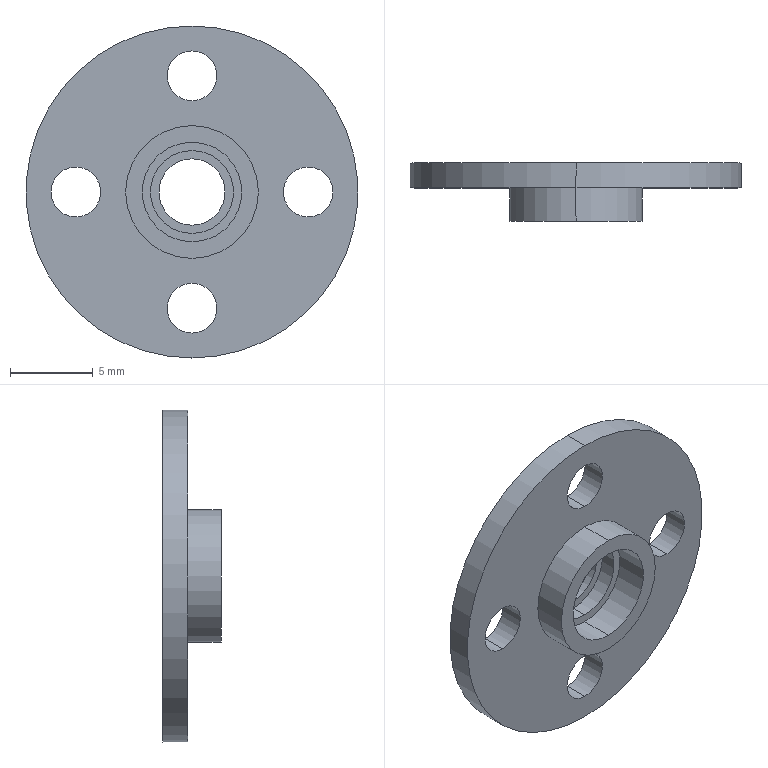Part | SolidWorks | features ICE 1, Revolution 1 | 1 solid | 23 faces | box 20 x 3.5 x 20 mm | volume 446.892 mm3 | cylinder 18 | plane 5 | commonest cylinder face diameters 3 x8 4 x2 5 x2 6 x2 8 x2 20 x2
STEP:
#1=CARTESIAN_POINT('',(4.861,-0.2196,-1.5));
#2=VERTEX_POINT('',#1);
#3=CARTESIAN_POINT('',(4.861,-0.2196,1.5));
#4=VERTEX_POINT('',#3);
#5=CARTESIAN_POINT('',(4.861,-0.2196,0.));
#6=DIRECTION('',(0.,1.,0.));
#7=DIRECTION('',(0.,0.,1.));
#8=AXIS2_PLACEMENT_3D('',#5,#6,#7);
#9=CIRCLE('',#8,1.5);
#10=EDGE_CURVE('',#2,#4,#9,.T.);
#11=ORIENTED_EDGE('',*,*,#10,.F.);
#12=CARTESIAN_POINT('',(4.861,1.28,-1.5));
#13=VERTEX_POINT('',#12);
#14=CARTESIAN_POINT('',(4.861,-8.72,-1.5));
#15=DIRECTION('',(0.,1.,0.));
#16=VECTOR('',#15,1000.);
#17=LINE('',#14,#16);
#18=EDGE_CURVE('',#2,#13,#17,.T.);
#19=ORIENTED_EDGE('',*,*,#18,.T.);
#20=CARTESIAN_POINT('',(4.861,1.28,1.5));
#21=VERTEX_POINT('',#20);
#22=CARTESIAN_POINT('',(4.861,1.28,0.));
#23=DIRECTION('',(0.,1.,0.));
#24=DIRECTION('',(0.,0.,1.));
#25=AXIS2_PLACEMENT_3D('',#22,#23,#24);
#26=CIRCLE('',#25,1.5);
#27=EDGE_CURVE('',#13,#21,#26,.T.);
#28=ORIENTED_EDGE('',*,*,#27,.T.);
#29=CARTESIAN_POINT('',(4.861,-8.72,1.5));
#30=DIRECTION('',(0.,1.,0.));
#31=VECTOR('',#30,1000.);
#32=LINE('',#29,#31);
#33=EDGE_CURVE('',#4,#21,#32,.T.);
#34=ORIENTED_EDGE('',*,*,#33,.F.);
#35=EDGE_LOOP('',(#11,#19,#28,#34));
#36=FACE_OUTER_BOUND('',#35,.T.);
#37=CARTESIAN_POINT('',(4.861,-8.72,0.));
#38=DIRECTION('',(0.,1.,0.));
#39=DIRECTION('',(0.,0.,1.));
#40=AXIS2_PLACEMENT_3D('',#37,#38,#39);
#41=CYLINDRICAL_SURFACE('',#40,1.5);
#42=ADVANCED_FACE('',(#36),#41,.F.);
#43=CARTESIAN_POINT('',(-2.139,-0.2196,-8.5));
#44=VERTEX_POINT('',#43);
#45=CARTESIAN_POINT('',(-2.139,-0.2196,-5.5));
#46=VERTEX_POINT('',#45);
#47=CARTESIAN_POINT('',(-2.139,-0.2196,-7.));
#48=DIRECTION('',(0.,1.,0.));
#49=DIRECTION('',(0.,0.,1.));
#50=AXIS2_PLACEMENT_3D('',#47,#48,#49);
#51=CIRCLE('',#50,1.5);
#52=EDGE_CURVE('',#44,#46,#51,.T.);
#53=ORIENTED_EDGE('',*,*,#52,.F.);
#54=CARTESIAN_POINT('',(-2.139,1.28,-8.5));
#55=VERTEX_POINT('',#54);
#56=CARTESIAN_POINT('',(-2.139,-8.72,-8.5));
#57=DIRECTION('',(0.,1.,0.));
#58=VECTOR('',#57,1000.);
#59=LINE('',#56,#58);
#60=EDGE_CURVE('',#44,#55,#59,.T.);
#61=ORIENTED_EDGE('',*,*,#60,.T.);
#62=CARTESIAN_POINT('',(-2.139,1.28,-5.5));
#63=VERTEX_POINT('',#62);
#64=CARTESIAN_POINT('',(-2.139,1.28,-7.));
#65=DIRECTION('',(0.,1.,0.));
#66=DIRECTION('',(0.,0.,1.));
#67=AXIS2_PLACEMENT_3D('',#64,#65,#66);
#68=CIRCLE('',#67,1.5);
#69=EDGE_CURVE('',#55,#63,#68,.T.);
#70=ORIENTED_EDGE('',*,*,#69,.T.);
#71=CARTESIAN_POINT('',(-2.139,-8.72,-5.5));
#72=DIRECTION('',(0.,1.,0.));
#73=VECTOR('',#72,1000.);
#74=LINE('',#71,#73);
#75=EDGE_CURVE('',#46,#63,#74,.T.);
#76=ORIENTED_EDGE('',*,*,#75,.F.);
#77=EDGE_LOOP('',(#53,#61,#70,#76));
#78=FACE_OUTER_BOUND('',#77,.T.);
#79=CARTESIAN_POINT('',(-2.139,-8.72,-7.));
#80=DIRECTION('',(0.,1.,0.));
#81=DIRECTION('',(0.,0.,1.));
#82=AXIS2_PLACEMENT_3D('',#79,#80,#81);
#83=CYLINDRICAL_SURFACE('',#82,1.5);
#84=ADVANCED_FACE('',(#78),#83,.F.);
#85=CARTESIAN_POINT('',(-2.139,-0.2196,5.5));
#86=VERTEX_POINT('',#85);
#87=CARTESIAN_POINT('',(-2.139,-0.2196,8.5));
#88=VERTEX_POINT('',#87);
#89=CARTESIAN_POINT('',(-2.139,-0.2196,7.));
#90=DIRECTION('',(0.,1.,0.));
#91=DIRECTION('',(0.,0.,1.));
#92=AXIS2_PLACEMENT_3D('',#89,#90,#91);
#93=CIRCLE('',#92,1.5);
#94=EDGE_CURVE('',#86,#88,#93,.T.);
#95=ORIENTED_EDGE('',*,*,#94,.F.);
#96=CARTESIAN_POINT('',(-2.139,1.28,5.5));
#97=VERTEX_POINT('',#96);
#98=CARTESIAN_POINT('',(-2.139,-8.72,5.5));
#99=DIRECTION('',(0.,1.,0.));
#100=VECTOR('',#99,1000.);
#101=LINE('',#98,#100);
#102=EDGE_CURVE('',#86,#97,#101,.T.);
#103=ORIENTED_EDGE('',*,*,#102,.T.);
#104=CARTESIAN_POINT('',(-2.139,1.28,8.5));
#105=VERTEX_POINT('',#104);
#106=CARTESIAN_POINT('',(-2.139,1.28,7.));
#107=DIRECTION('',(0.,1.,0.));
#108=DIRECTION('',(0.,0.,1.));
#109=AXIS2_PLACEMENT_3D('',#106,#107,#108);
#110=CIRCLE('',#109,1.5);
#111=EDGE_CURVE('',#97,#105,#110,.T.);
#112=ORIENTED_EDGE('',*,*,#111,.T.);
#113=CARTESIAN_POINT('',(-2.139,-8.72,8.5));
#114=DIRECTION('',(0.,1.,0.));
#115=VECTOR('',#114,1000.);
#116=LINE('',#113,#115);
#117=EDGE_CURVE('',#88,#105,#116,.T.);
#118=ORIENTED_EDGE('',*,*,#117,.F.);
#119=EDGE_LOOP('',(#95,#103,#112,#118));
#120=FACE_OUTER_BOUND('',#119,.T.);
#121=CARTESIAN_POINT('',(-2.139,-8.72,7.));
#122=DIRECTION('',(0.,1.,0.));
#123=DIRECTION('',(0.,0.,1.));
#124=AXIS2_PLACEMENT_3D('',#121,#122,#123);
#125=CYLINDRICAL_SURFACE('',#124,1.5);
#126=ADVANCED_FACE('',(#120),#125,.F.);
#127=CARTESIAN_POINT('',(-9.139,-0.2196,-1.5));
#128=VERTEX_POINT('',#127);
#129=CARTESIAN_POINT('',(-9.139,-0.2196,1.5));
#130=VERTEX_POINT('',#129);
#131=CARTESIAN_POINT('',(-9.139,-0.2196,0.));
#132=DIRECTION('',(0.,1.,0.));
#133=DIRECTION('',(0.,0.,1.));
#134=AXIS2_PLACEMENT_3D('',#131,#132,#133);
#135=CIRCLE('',#134,1.5);
#136=EDGE_CURVE('',#128,#130,#135,.T.);
#137=ORIENTED_EDGE('',*,*,#136,.F.);
#138=CARTESIAN_POINT('',(-9.139,1.28,-1.5));
#139=VERTEX_POINT('',#138);
#140=CARTESIAN_POINT('',(-9.139,-8.72,-1.5));
#141=DIRECTION('',(0.,1.,0.));
#142=VECTOR('',#141,1000.);
#143=LINE('',#140,#142);
#144=EDGE_CURVE('',#128,#139,#143,.T.);
#145=ORIENTED_EDGE('',*,*,#144,.T.);
#146=CARTESIAN_POINT('',(-9.139,1.28,1.5));
#147=VERTEX_POINT('',#146);
#148=CARTESIAN_POINT('',(-9.139,1.28,0.));
#149=DIRECTION('',(0.,1.,0.));
#150=DIRECTION('',(0.,0.,1.));
#151=AXIS2_PLACEMENT_3D('',#148,#149,#150);
#152=CIRCLE('',#151,1.5);
#153=EDGE_CURVE('',#139,#147,#152,.T.);
#154=ORIENTED_EDGE('',*,*,#153,.T.);
#155=CARTESIAN_POINT('',(-9.139,-8.72,1.5));
#156=DIRECTION('',(0.,1.,0.));
#157=VECTOR('',#156,1000.);
#158=LINE('',#155,#157);
#159=EDGE_CURVE('',#130,#147,#158,.T.);
#160=ORIENTED_EDGE('',*,*,#159,.F.);
#161=EDGE_LOOP('',(#137,#145,#154,#160));
#162=FACE_OUTER_BOUND('',#161,.T.);
#163=CARTESIAN_POINT('',(-9.139,-8.72,0.));
#164=DIRECTION('',(0.,1.,0.));
#165=DIRECTION('',(0.,0.,1.));
#166=AXIS2_PLACEMENT_3D('',#163,#164,#165);
#167=CYLINDRICAL_SURFACE('',#166,1.5);
#168=ADVANCED_FACE('',(#162),#167,.F.);
#169=CARTESIAN_POINT('',(-2.139,-0.2196,-2.5));
#170=VERTEX_POINT('',#169);
#171=CARTESIAN_POINT('',(-2.139,-0.2196,2.5));
#172=VERTEX_POINT('',#171);
#173=CARTESIAN_POINT('',(-2.139,-0.2196,0.));
#174=DIRECTION('',(0.,1.,0.));
#175=DIRECTION('',(0.,0.,1.));
#176=AXIS2_PLACEMENT_3D('',#173,#174,#175);
#177=CIRCLE('',#176,2.5);
#178=EDGE_CURVE('',#170,#172,#177,.T.);
#179=ORIENTED_EDGE('',*,*,#178,.F.);
#180=CARTESIAN_POINT('',(-2.139,0.7804,-2.5));
#181=VERTEX_POINT('',#180);
#182=CARTESIAN_POINT('',(-2.139,1.541,-2.5));
#183=DIRECTION('',(0.,1.,0.));
#184=VECTOR('',#183,1000.);
#185=LINE('',#182,#184);
#186=EDGE_CURVE('',#170,#181,#185,.T.);
#187=ORIENTED_EDGE('',*,*,#186,.T.);
#188=CARTESIAN_POINT('',(-2.139,0.7804,2.5));
#189=VERTEX_POINT('',#188);
#190=CARTESIAN_POINT('',(-2.139,0.7804,0.));
#191=DIRECTION('',(0.,1.,0.));
#192=DIRECTION('',(0.,0.,1.));
#193=AXIS2_PLACEMENT_3D('',#190,#191,#192);
#194=CIRCLE('',#193,2.5);
#195=EDGE_CURVE('',#181,#189,#194,.T.);
#196=ORIENTED_EDGE('',*,*,#195,.T.);
#197=CARTESIAN_POINT('',(-2.139,1.541,2.5));
#198=DIRECTION('',(0.,1.,0.));
#199=VECTOR('',#198,1000.);
#200=LINE('',#197,#199);
#201=EDGE_CURVE('',#172,#189,#200,.T.);
#202=ORIENTED_EDGE('',*,*,#201,.F.);
#203=EDGE_LOOP('',(#179,#187,#196,#202));
#204=FACE_OUTER_BOUND('',#203,.T.);
#205=CARTESIAN_POINT('',(-2.139,1.541,0.));
#206=DIRECTION('',(0.,1.,0.));
#207=DIRECTION('',(0.,0.,1.));
#208=AXIS2_PLACEMENT_3D('',#205,#206,#207);
#209=CYLINDRICAL_SURFACE('',#208,2.5);
#210=ADVANCED_FACE('',(#204),#209,.F.);
#211=CARTESIAN_POINT('',(-2.139,-2.22,-3.));
#212=VERTEX_POINT('',#211);
#213=CARTESIAN_POINT('',(-2.139,-2.22,3.));
#214=VERTEX_POINT('',#213);
#215=CARTESIAN_POINT('',(-2.139,-2.22,0.));
#216=DIRECTION('',(0.,1.,0.));
#217=DIRECTION('',(0.,0.,1.));
#218=AXIS2_PLACEMENT_3D('',#215,#216,#217);
#219=CIRCLE('',#218,3.);
#220=EDGE_CURVE('',#212,#214,#219,.T.);
#221=ORIENTED_EDGE('',*,*,#220,.F.);
#222=CARTESIAN_POINT('',(-2.139,-0.2196,-3.));
#223=VERTEX_POINT('',#222);
#224=CARTESIAN_POINT('',(-2.139,1.541,-3.));
#225=DIRECTION('',(0.,1.,0.));
#226=VECTOR('',#225,1000.);
#227=LINE('',#224,#226);
#228=EDGE_CURVE('',#212,#223,#227,.T.);
#229=ORIENTED_EDGE('',*,*,#228,.T.);
#230=CARTESIAN_POINT('',(-2.139,-0.2196,3.));
#231=VERTEX_POINT('',#230);
#232=CARTESIAN_POINT('',(-2.139,-0.2196,0.));
#233=DIRECTION('',(0.,1.,0.));
#234=DIRECTION('',(0.,0.,1.));
#235=AXIS2_PLACEMENT_3D('',#232,#233,#234);
#236=CIRCLE('',#235,3.);
#237=EDGE_CURVE('',#223,#231,#236,.T.);
#238=ORIENTED_EDGE('',*,*,#237,.T.);
#239=CARTESIAN_POINT('',(-2.139,1.541,3.));
#240=DIRECTION('',(0.,1.,0.));
#241=VECTOR('',#240,1000.);
#242=LINE('',#239,#241);
#243=EDGE_CURVE('',#214,#231,#242,.T.);
#244=ORIENTED_EDGE('',*,*,#243,.F.);
#245=EDGE_LOOP('',(#221,#229,#238,#244));
#246=FACE_OUTER_BOUND('',#245,.T.);
#247=CARTESIAN_POINT('',(-2.139,1.541,0.));
#248=DIRECTION('',(0.,1.,0.));
#249=DIRECTION('',(0.,0.,1.));
#250=AXIS2_PLACEMENT_3D('',#247,#248,#249);
#251=CYLINDRICAL_SURFACE('',#250,3.);
#252=ADVANCED_FACE('',(#246),#251,.F.);
#253=CARTESIAN_POINT('',(-2.139,-2.22,4.));
#254=VERTEX_POINT('',#253);
#255=CARTESIAN_POINT('',(-2.139,-2.22,-4.));
#256=VERTEX_POINT('',#255);
#257=CARTESIAN_POINT('',(-2.139,-2.22,0.));
#258=DIRECTION('',(0.,1.,0.));
#259=DIRECTION('',(0.,0.,1.));
#260=AXIS2_PLACEMENT_3D('',#257,#258,#259);
#261=CIRCLE('',#260,4.);
#262=EDGE_CURVE('',#254,#256,#261,.T.);
#263=ORIENTED_EDGE('',*,*,#262,.T.);
#264=CARTESIAN_POINT('',(-2.139,-0.2196,-4.));
#265=VERTEX_POINT('',#264);
#266=CARTESIAN_POINT('',(-2.139,1.541,-4.));
#267=DIRECTION('',(0.,1.,0.));
#268=VECTOR('',#267,1000.);
#269=LINE('',#266,#268);
#270=EDGE_CURVE('',#256,#265,#269,.T.);
#271=ORIENTED_EDGE('',*,*,#270,.T.);
#272=CARTESIAN_POINT('',(-2.139,-0.2196,4.));
#273=VERTEX_POINT('',#272);
#274=CARTESIAN_POINT('',(-2.139,-0.2196,0.));
#275=DIRECTION('',(0.,1.,0.));
#276=DIRECTION('',(0.,0.,1.));
#277=AXIS2_PLACEMENT_3D('',#274,#275,#276);
#278=CIRCLE('',#277,4.);
#279=EDGE_CURVE('',#273,#265,#278,.T.);
#280=ORIENTED_EDGE('',*,*,#279,.F.);
#281=CARTESIAN_POINT('',(-2.139,1.541,4.));
#282=DIRECTION('',(0.,1.,0.));
#283=VECTOR('',#282,1000.);
#284=LINE('',#281,#283);
#285=EDGE_CURVE('',#254,#273,#284,.T.);
#286=ORIENTED_EDGE('',*,*,#285,.F.);
#287=EDGE_LOOP('',(#263,#271,#280,#286));
#288=FACE_OUTER_BOUND('',#287,.T.);
#289=CARTESIAN_POINT('',(-2.139,1.541,0.));
#290=DIRECTION('',(0.,1.,0.));
#291=DIRECTION('',(0.,0.,1.));
#292=AXIS2_PLACEMENT_3D('',#289,#290,#291);
#293=CYLINDRICAL_SURFACE('',#292,4.);
#294=ADVANCED_FACE('',(#288),#293,.T.);
#295=CARTESIAN_POINT('',(-2.139,-0.2196,10.));
#296=VERTEX_POINT('',#295);
#297=CARTESIAN_POINT('',(-2.139,-0.2196,-10.));
#298=VERTEX_POINT('',#297);
#299=CARTESIAN_POINT('',(-2.139,-0.2196,0.));
#300=DIRECTION('',(0.,1.,0.));
#301=DIRECTION('',(0.,0.,1.));
#302=AXIS2_PLACEMENT_3D('',#299,#300,#301);
#303=CIRCLE('',#302,10.);
#304=EDGE_CURVE('',#296,#298,#303,.T.);
#305=ORIENTED_EDGE('',*,*,#304,.T.);
#306=CARTESIAN_POINT('',(-2.139,1.28,-10.));
#307=VERTEX_POINT('',#306);
#308=CARTESIAN_POINT('',(-2.139,1.541,-10.));
#309=DIRECTION('',(0.,1.,0.));
#310=VECTOR('',#309,1000.);
#311=LINE('',#308,#310);
#312=EDGE_CURVE('',#298,#307,#311,.T.);
#313=ORIENTED_EDGE('',*,*,#312,.T.);
#314=CARTESIAN_POINT('',(-2.139,1.28,10.));
#315=VERTEX_POINT('',#314);
#316=CARTESIAN_POINT('',(-2.139,1.28,0.));
#317=DIRECTION('',(0.,1.,0.));
#318=DIRECTION('',(0.,0.,1.));
#319=AXIS2_PLACEMENT_3D('',#316,#317,#318);
#320=CIRCLE('',#319,10.);
#321=EDGE_CURVE('',#315,#307,#320,.T.);
#322=ORIENTED_EDGE('',*,*,#321,.F.);
#323=CARTESIAN_POINT('',(-2.139,1.541,10.));
#324=DIRECTION('',(0.,1.,0.));
#325=VECTOR('',#324,1000.);
#326=LINE('',#323,#325);
#327=EDGE_CURVE('',#296,#315,#326,.T.);
#328=ORIENTED_EDGE('',*,*,#327,.F.);
#329=EDGE_LOOP('',(#305,#313,#322,#328));
#330=FACE_OUTER_BOUND('',#329,.T.);
#331=CARTESIAN_POINT('',(-2.139,1.541,0.));
#332=DIRECTION('',(0.,1.,0.));
#333=DIRECTION('',(0.,0.,1.));
#334=AXIS2_PLACEMENT_3D('',#331,#332,#333);
#335=CYLINDRICAL_SURFACE('',#334,10.);
#336=ADVANCED_FACE('',(#330),#335,.T.);
#337=CARTESIAN_POINT('',(-2.139,0.7804,-2.));
#338=VERTEX_POINT('',#337);
#339=CARTESIAN_POINT('',(-2.139,0.7804,2.));
#340=VERTEX_POINT('',#339);
#341=CARTESIAN_POINT('',(-2.139,0.7804,0.));
#342=DIRECTION('',(0.,1.,0.));
#343=DIRECTION('',(0.,0.,1.));
#344=AXIS2_PLACEMENT_3D('',#341,#342,#343);
#345=CIRCLE('',#344,2.);
#346=EDGE_CURVE('',#338,#340,#345,.T.);
#347=ORIENTED_EDGE('',*,*,#346,.F.);
#348=CARTESIAN_POINT('',(-2.139,1.28,-2.));
#349=VERTEX_POINT('',#348);
#350=CARTESIAN_POINT('',(-2.139,1.541,-2.));
#351=DIRECTION('',(0.,1.,0.));
#352=VECTOR('',#351,1000.);
#353=LINE('',#350,#352);
#354=EDGE_CURVE('',#338,#349,#353,.T.);
#355=ORIENTED_EDGE('',*,*,#354,.T.);
#356=CARTESIAN_POINT('',(-2.139,1.28,2.));
#357=VERTEX_POINT('',#356);
#358=CARTESIAN_POINT('',(-2.139,1.28,0.));
#359=DIRECTION('',(0.,1.,0.));
#360=DIRECTION('',(0.,0.,1.));
#361=AXIS2_PLACEMENT_3D('',#358,#359,#360);
#362=CIRCLE('',#361,2.);
#363=EDGE_CURVE('',#349,#357,#362,.T.);
#364=ORIENTED_EDGE('',*,*,#363,.T.);
#365=CARTESIAN_POINT('',(-2.139,1.541,2.));
#366=DIRECTION('',(0.,1.,0.));
#367=VECTOR('',#366,1000.);
#368=LINE('',#365,#367);
#369=EDGE_CURVE('',#340,#357,#368,.T.);
#370=ORIENTED_EDGE('',*,*,#369,.F.);
#371=EDGE_LOOP('',(#347,#355,#364,#370));
#372=FACE_OUTER_BOUND('',#371,.T.);
#373=CARTESIAN_POINT('',(-2.139,1.541,0.));
#374=DIRECTION('',(0.,1.,0.));
#375=DIRECTION('',(0.,0.,1.));
#376=AXIS2_PLACEMENT_3D('',#373,#374,#375);
#377=CYLINDRICAL_SURFACE('',#376,2.);
#378=ADVANCED_FACE('',(#372),#377,.F.);
#379=ORIENTED_EDGE('',*,*,#354,.F.);
#380=CARTESIAN_POINT('',(-2.139,0.7804,0.));
#381=DIRECTION('',(0.,1.,0.));
#382=DIRECTION('',(0.,0.,1.));
#383=AXIS2_PLACEMENT_3D('',#380,#381,#382);
#384=CIRCLE('',#383,2.);
#385=EDGE_CURVE('',#340,#338,#384,.T.);
#386=ORIENTED_EDGE('',*,*,#385,.F.);
#387=ORIENTED_EDGE('',*,*,#369,.T.);
#388=CARTESIAN_POINT('',(-2.139,1.28,0.));
#389=DIRECTION('',(0.,1.,0.));
#390=DIRECTION('',(0.,0.,1.));
#391=AXIS2_PLACEMENT_3D('',#388,#389,#390);
#392=CIRCLE('',#391,2.);
#393=EDGE_CURVE('',#357,#349,#392,.T.);
#394=ORIENTED_EDGE('',*,*,#393,.T.);
#395=EDGE_LOOP('',(#379,#386,#387,#394));
#396=FACE_OUTER_BOUND('',#395,.T.);
#397=CARTESIAN_POINT('',(-2.139,1.541,0.));
#398=DIRECTION('',(0.,1.,0.));
#399=DIRECTION('',(0.,0.,1.));
#400=AXIS2_PLACEMENT_3D('',#397,#398,#399);
#401=CYLINDRICAL_SURFACE('',#400,2.);
#402=ADVANCED_FACE('',(#396),#401,.F.);
#403=CARTESIAN_POINT('',(4.861,1.28,0.));
#404=DIRECTION('',(0.,1.,0.));
#405=DIRECTION('',(0.,0.,1.));
#406=AXIS2_PLACEMENT_3D('',#403,#404,#405);
#407=CIRCLE('',#406,1.5);
#408=EDGE_CURVE('',#21,#13,#407,.T.);
#409=ORIENTED_EDGE('',*,*,#408,.F.);
#410=ORIENTED_EDGE('',*,*,#27,.F.);
#411=EDGE_LOOP('',(#409,#410));
#412=FACE_BOUND('',#411,.T.);
#413=CARTESIAN_POINT('',(-2.139,1.28,-7.));
#414=DIRECTION('',(0.,1.,0.));
#415=DIRECTION('',(0.,0.,1.));
#416=AXIS2_PLACEMENT_3D('',#413,#414,#415);
#417=CIRCLE('',#416,1.5);
#418=EDGE_CURVE('',#63,#55,#417,.T.);
#419=ORIENTED_EDGE('',*,*,#418,.F.);
#420=ORIENTED_EDGE('',*,*,#69,.F.);
#421=EDGE_LOOP('',(#419,#420));
#422=FACE_BOUND('',#421,.T.);
#423=CARTESIAN_POINT('',(-2.139,1.28,7.));
#424=DIRECTION('',(0.,1.,0.));
#425=DIRECTION('',(0.,0.,1.));
#426=AXIS2_PLACEMENT_3D('',#423,#424,#425);
#427=CIRCLE('',#426,1.5);
#428=EDGE_CURVE('',#105,#97,#427,.T.);
#429=ORIENTED_EDGE('',*,*,#428,.F.);
#430=ORIENTED_EDGE('',*,*,#111,.F.);
#431=EDGE_LOOP('',(#429,#430));
#432=FACE_BOUND('',#431,.T.);
#433=CARTESIAN_POINT('',(-9.139,1.28,0.));
#434=DIRECTION('',(0.,1.,0.));
#435=DIRECTION('',(0.,0.,1.));
#436=AXIS2_PLACEMENT_3D('',#433,#434,#435);
#437=CIRCLE('',#436,1.5);
#438=EDGE_CURVE('',#147,#139,#437,.T.);
#439=ORIENTED_EDGE('',*,*,#438,.F.);
#440=ORIENTED_EDGE('',*,*,#153,.F.);
#441=EDGE_LOOP('',(#439,#440));
#442=FACE_BOUND('',#441,.T.);
#443=ORIENTED_EDGE('',*,*,#393,.F.);
#444=ORIENTED_EDGE('',*,*,#363,.F.);
#445=EDGE_LOOP('',(#443,#444));
#446=FACE_BOUND('',#445,.T.);
#447=ORIENTED_EDGE('',*,*,#321,.T.);
#448=CARTESIAN_POINT('',(-2.139,1.28,0.));
#449=DIRECTION('',(0.,1.,0.));
#450=DIRECTION('',(0.,0.,1.));
#451=AXIS2_PLACEMENT_3D('',#448,#449,#450);
#452=CIRCLE('',#451,10.);
#453=EDGE_CURVE('',#307,#315,#452,.T.);
#454=ORIENTED_EDGE('',*,*,#453,.T.);
#455=EDGE_LOOP('',(#447,#454));
#456=FACE_OUTER_BOUND('',#455,.T.);
#457=CARTESIAN_POINT('',(-0.1385,1.28,0.));
#458=DIRECTION('',(0.,-1.,0.));
#459=DIRECTION('',(0.,0.,-1.));
#460=AXIS2_PLACEMENT_3D('',#457,#458,#459);
#461=PLANE('',#460);
#462=ADVANCED_FACE('',(#412,#422,#432,#442,#446,#456),#461,.F.);
#463=ORIENTED_EDGE('',*,*,#312,.F.);
#464=CARTESIAN_POINT('',(-2.139,-0.2196,0.));
#465=DIRECTION('',(0.,1.,0.));
#466=DIRECTION('',(0.,0.,1.));
#467=AXIS2_PLACEMENT_3D('',#464,#465,#466);
#468=CIRCLE('',#467,10.);
#469=EDGE_CURVE('',#298,#296,#468,.T.);
#470=ORIENTED_EDGE('',*,*,#469,.T.);
#471=ORIENTED_EDGE('',*,*,#327,.T.);
#472=ORIENTED_EDGE('',*,*,#453,.F.);
#473=EDGE_LOOP('',(#463,#470,#471,#472));
#474=FACE_OUTER_BOUND('',#473,.T.);
#475=CARTESIAN_POINT('',(-2.139,1.541,0.));
#476=DIRECTION('',(0.,1.,0.));
#477=DIRECTION('',(0.,0.,1.));
#478=AXIS2_PLACEMENT_3D('',#475,#476,#477);
#479=CYLINDRICAL_SURFACE('',#478,10.);
#480=ADVANCED_FACE('',(#474),#479,.T.);
#481=CARTESIAN_POINT('',(4.861,-0.2196,0.));
#482=DIRECTION('',(0.,1.,0.));
#483=DIRECTION('',(0.,0.,1.));
#484=AXIS2_PLACEMENT_3D('',#481,#482,#483);
#485=CIRCLE('',#484,1.5);
#486=EDGE_CURVE('',#4,#2,#485,.T.);
#487=ORIENTED_EDGE('',*,*,#486,.T.);
#488=ORIENTED_EDGE('',*,*,#10,.T.);
#489=EDGE_LOOP('',(#487,#488));
#490=FACE_BOUND('',#489,.T.);
#491=CARTESIAN_POINT('',(-2.139,-0.2196,-7.));
#492=DIRECTION('',(0.,1.,0.));
#493=DIRECTION('',(0.,0.,1.));
#494=AXIS2_PLACEMENT_3D('',#491,#492,#493);
#495=CIRCLE('',#494,1.5);
#496=EDGE_CURVE('',#46,#44,#495,.T.);
#497=ORIENTED_EDGE('',*,*,#496,.T.);
#498=ORIENTED_EDGE('',*,*,#52,.T.);
#499=EDGE_LOOP('',(#497,#498));
#500=FACE_BOUND('',#499,.T.);
#501=CARTESIAN_POINT('',(-2.139,-0.2196,7.));
#502=DIRECTION('',(0.,1.,0.));
#503=DIRECTION('',(0.,0.,1.));
#504=AXIS2_PLACEMENT_3D('',#501,#502,#503);
#505=CIRCLE('',#504,1.5);
#506=EDGE_CURVE('',#88,#86,#505,.T.);
#507=ORIENTED_EDGE('',*,*,#506,.T.);
#508=ORIENTED_EDGE('',*,*,#94,.T.);
#509=EDGE_LOOP('',(#507,#508));
#510=FACE_BOUND('',#509,.T.);
#511=CARTESIAN_POINT('',(-9.139,-0.2196,0.));
#512=DIRECTION('',(0.,1.,0.));
#513=DIRECTION('',(0.,0.,1.));
#514=AXIS2_PLACEMENT_3D('',#511,#512,#513);
#515=CIRCLE('',#514,1.5);
#516=EDGE_CURVE('',#130,#128,#515,.T.);
#517=ORIENTED_EDGE('',*,*,#516,.T.);
#518=ORIENTED_EDGE('',*,*,#136,.T.);
#519=EDGE_LOOP('',(#517,#518));
#520=FACE_BOUND('',#519,.T.);
#521=ORIENTED_EDGE('',*,*,#304,.F.);
#522=ORIENTED_EDGE('',*,*,#469,.F.);
#523=EDGE_LOOP('',(#521,#522));
#524=FACE_OUTER_BOUND('',#523,.T.);
#525=ORIENTED_EDGE('',*,*,#279,.T.);
#526=CARTESIAN_POINT('',(-2.139,-0.2196,0.));
#527=DIRECTION('',(0.,1.,0.));
#528=DIRECTION('',(0.,0.,1.));
#529=AXIS2_PLACEMENT_3D('',#526,#527,#528);
#530=CIRCLE('',#529,4.);
#531=EDGE_CURVE('',#265,#273,#530,.T.);
#532=ORIENTED_EDGE('',*,*,#531,.T.);
#533=EDGE_LOOP('',(#525,#532));
#534=FACE_BOUND('',#533,.T.);
#535=CARTESIAN_POINT('',(7.861,-0.2196,0.));
#536=DIRECTION('',(0.,1.,0.));
#537=DIRECTION('',(0.,0.,1.));
#538=AXIS2_PLACEMENT_3D('',#535,#536,#537);
#539=PLANE('',#538);
#540=ADVANCED_FACE('',(#490,#500,#510,#520,#524,#534),#539,.F.);
#541=ORIENTED_EDGE('',*,*,#270,.F.);
#542=CARTESIAN_POINT('',(-2.139,-2.22,0.));
#543=DIRECTION('',(0.,1.,0.));
#544=DIRECTION('',(0.,0.,1.));
#545=AXIS2_PLACEMENT_3D('',#542,#543,#544);
#546=CIRCLE('',#545,4.);
#547=EDGE_CURVE('',#256,#254,#546,.T.);
#548=ORIENTED_EDGE('',*,*,#547,.T.);
#549=ORIENTED_EDGE('',*,*,#285,.T.);
#550=ORIENTED_EDGE('',*,*,#531,.F.);
#551=EDGE_LOOP('',(#541,#548,#549,#550));
#552=FACE_OUTER_BOUND('',#551,.T.);
#553=CARTESIAN_POINT('',(-2.139,1.541,0.));
#554=DIRECTION('',(0.,1.,0.));
#555=DIRECTION('',(0.,0.,1.));
#556=AXIS2_PLACEMENT_3D('',#553,#554,#555);
#557=CYLINDRICAL_SURFACE('',#556,4.);
#558=ADVANCED_FACE('',(#552),#557,.T.);
#559=ORIENTED_EDGE('',*,*,#262,.F.);
#560=ORIENTED_EDGE('',*,*,#547,.F.);
#561=EDGE_LOOP('',(#559,#560));
#562=FACE_OUTER_BOUND('',#561,.T.);
#563=CARTESIAN_POINT('',(-2.139,-2.22,0.));
#564=DIRECTION('',(0.,1.,0.));
#565=DIRECTION('',(0.,0.,1.));
#566=AXIS2_PLACEMENT_3D('',#563,#564,#565);
#567=CIRCLE('',#566,3.);
#568=EDGE_CURVE('',#214,#212,#567,.T.);
#569=ORIENTED_EDGE('',*,*,#568,.T.);
#570=ORIENTED_EDGE('',*,*,#220,.T.);
#571=EDGE_LOOP('',(#569,#570));
#572=FACE_BOUND('',#571,.T.);
#573=CARTESIAN_POINT('',(1.861,-2.22,0.));
#574=DIRECTION('',(0.,1.,0.));
#575=DIRECTION('',(0.,0.,1.));
#576=AXIS2_PLACEMENT_3D('',#573,#574,#575);
#577=PLANE('',#576);
#578=ADVANCED_FACE('',(#562,#572),#577,.F.);
#579=ORIENTED_EDGE('',*,*,#228,.F.);
#580=ORIENTED_EDGE('',*,*,#568,.F.);
#581=ORIENTED_EDGE('',*,*,#243,.T.);
#582=CARTESIAN_POINT('',(-2.139,-0.2196,0.));
#583=DIRECTION('',(0.,1.,0.));
#584=DIRECTION('',(0.,0.,1.));
#585=AXIS2_PLACEMENT_3D('',#582,#583,#584);
#586=CIRCLE('',#585,3.);
#587=EDGE_CURVE('',#231,#223,#586,.T.);
#588=ORIENTED_EDGE('',*,*,#587,.T.);
#589=EDGE_LOOP('',(#579,#580,#581,#588));
#590=FACE_OUTER_BOUND('',#589,.T.);
#591=CARTESIAN_POINT('',(-2.139,1.541,0.));
#592=DIRECTION('',(0.,1.,0.));
#593=DIRECTION('',(0.,0.,1.));
#594=AXIS2_PLACEMENT_3D('',#591,#592,#593);
#595=CYLINDRICAL_SURFACE('',#594,3.);
#596=ADVANCED_FACE('',(#590),#595,.F.);
#597=ORIENTED_EDGE('',*,*,#587,.F.);
#598=ORIENTED_EDGE('',*,*,#237,.F.);
#599=EDGE_LOOP('',(#597,#598));
#600=FACE_OUTER_BOUND('',#599,.T.);
#601=CARTESIAN_POINT('',(-2.139,-0.2196,0.));
#602=DIRECTION('',(0.,1.,0.));
#603=DIRECTION('',(0.,0.,1.));
#604=AXIS2_PLACEMENT_3D('',#601,#602,#603);
#605=CIRCLE('',#604,2.5);
#606=EDGE_CURVE('',#172,#170,#605,.T.);
#607=ORIENTED_EDGE('',*,*,#606,.T.);
#608=ORIENTED_EDGE('',*,*,#178,.T.);
#609=EDGE_LOOP('',(#607,#608));
#610=FACE_BOUND('',#609,.T.);
#611=CARTESIAN_POINT('',(0.8615,-0.2196,0.));
#612=DIRECTION('',(0.,1.,0.));
#613=DIRECTION('',(0.,0.,1.));
#614=AXIS2_PLACEMENT_3D('',#611,#612,#613);
#615=PLANE('',#614);
#616=ADVANCED_FACE('',(#600,#610),#615,.F.);
#617=ORIENTED_EDGE('',*,*,#186,.F.);
#618=ORIENTED_EDGE('',*,*,#606,.F.);
#619=ORIENTED_EDGE('',*,*,#201,.T.);
#620=CARTESIAN_POINT('',(-2.139,0.7804,0.));
#621=DIRECTION('',(0.,1.,0.));
#622=DIRECTION('',(0.,0.,1.));
#623=AXIS2_PLACEMENT_3D('',#620,#621,#622);
#624=CIRCLE('',#623,2.5);
#625=EDGE_CURVE('',#189,#181,#624,.T.);
#626=ORIENTED_EDGE('',*,*,#625,.T.);
#627=EDGE_LOOP('',(#617,#618,#619,#626));
#628=FACE_OUTER_BOUND('',#627,.T.);
#629=CARTESIAN_POINT('',(-2.139,1.541,0.));
#630=DIRECTION('',(0.,1.,0.));
#631=DIRECTION('',(0.,0.,1.));
#632=AXIS2_PLACEMENT_3D('',#629,#630,#631);
#633=CYLINDRICAL_SURFACE('',#632,2.5);
#634=ADVANCED_FACE('',(#628),#633,.F.);
#635=ORIENTED_EDGE('',*,*,#625,.F.);
#636=ORIENTED_EDGE('',*,*,#195,.F.);
#637=EDGE_LOOP('',(#635,#636));
#638=FACE_OUTER_BOUND('',#637,.T.);
#639=ORIENTED_EDGE('',*,*,#385,.T.);
#640=ORIENTED_EDGE('',*,*,#346,.T.);
#641=EDGE_LOOP('',(#639,#640));
#642=FACE_BOUND('',#641,.T.);
#643=CARTESIAN_POINT('',(0.3615,0.7804,0.));
#644=DIRECTION('',(0.,1.,0.));
#645=DIRECTION('',(0.,0.,1.));
#646=AXIS2_PLACEMENT_3D('',#643,#644,#645);
#647=PLANE('',#646);
#648=ADVANCED_FACE('',(#638,#642),#647,.F.);
#649=ORIENTED_EDGE('',*,*,#144,.F.);
#650=ORIENTED_EDGE('',*,*,#516,.F.);
#651=ORIENTED_EDGE('',*,*,#159,.T.);
#652=ORIENTED_EDGE('',*,*,#438,.T.);
#653=EDGE_LOOP('',(#649,#650,#651,#652));
#654=FACE_OUTER_BOUND('',#653,.T.);
#655=CARTESIAN_POINT('',(-9.139,-8.72,0.));
#656=DIRECTION('',(0.,1.,0.));
#657=DIRECTION('',(0.,0.,1.));
#658=AXIS2_PLACEMENT_3D('',#655,#656,#657);
#659=CYLINDRICAL_SURFACE('',#658,1.5);
#660=ADVANCED_FACE('',(#654),#659,.F.);
#661=ORIENTED_EDGE('',*,*,#102,.F.);
#662=ORIENTED_EDGE('',*,*,#506,.F.);
#663=ORIENTED_EDGE('',*,*,#117,.T.);
#664=ORIENTED_EDGE('',*,*,#428,.T.);
#665=EDGE_LOOP('',(#661,#662,#663,#664));
#666=FACE_OUTER_BOUND('',#665,.T.);
#667=CARTESIAN_POINT('',(-2.139,-8.72,7.));
#668=DIRECTION('',(0.,1.,0.));
#669=DIRECTION('',(0.,0.,1.));
#670=AXIS2_PLACEMENT_3D('',#667,#668,#669);
#671=CYLINDRICAL_SURFACE('',#670,1.5);
#672=ADVANCED_FACE('',(#666),#671,.F.);
#673=ORIENTED_EDGE('',*,*,#60,.F.);
#674=ORIENTED_EDGE('',*,*,#496,.F.);
#675=ORIENTED_EDGE('',*,*,#75,.T.);
#676=ORIENTED_EDGE('',*,*,#418,.T.);
#677=EDGE_LOOP('',(#673,#674,#675,#676));
#678=FACE_OUTER_BOUND('',#677,.T.);
#679=CARTESIAN_POINT('',(-2.139,-8.72,-7.));
#680=DIRECTION('',(0.,1.,0.));
#681=DIRECTION('',(0.,0.,1.));
#682=AXIS2_PLACEMENT_3D('',#679,#680,#681);
#683=CYLINDRICAL_SURFACE('',#682,1.5);
#684=ADVANCED_FACE('',(#678),#683,.F.);
#685=ORIENTED_EDGE('',*,*,#18,.F.);
#686=ORIENTED_EDGE('',*,*,#486,.F.);
#687=ORIENTED_EDGE('',*,*,#33,.T.);
#688=ORIENTED_EDGE('',*,*,#408,.T.);
#689=EDGE_LOOP('',(#685,#686,#687,#688));
#690=FACE_OUTER_BOUND('',#689,.T.);
#691=CARTESIAN_POINT('',(4.861,-8.72,0.));
#692=DIRECTION('',(0.,1.,0.));
#693=DIRECTION('',(0.,0.,1.));
#694=AXIS2_PLACEMENT_3D('',#691,#692,#693);
#695=CYLINDRICAL_SURFACE('',#694,1.5);
#696=ADVANCED_FACE('',(#690),#695,.F.);
#697=CLOSED_SHELL('',(#42,#84,#126,#168,#210,#252,#294,#336,#378,#402,#462,#480,#540,#558,#578,#596,#616,#634,#648,#660,#672,#684,#696));
#698=MANIFOLD_SOLID_BREP('',#697);
#699=CARTESIAN_POINT('',(0.,0.,0.));
#700=DIRECTION('',(0.,0.,1.));
#701=DIRECTION('',(1.,0.,0.));
#702=AXIS2_PLACEMENT_3D('',#699,#700,#701);
#703=(LENGTH_UNIT()NAMED_UNIT(*)SI_UNIT(.MILLI.,.METRE.));
#704=UNCERTAINTY_MEASURE_WITH_UNIT(LENGTH_MEASURE(0.00001),#703,'','');
#705=(NAMED_UNIT(*)PLANE_ANGLE_UNIT()SI_UNIT($,.RADIAN.));
#706=(NAMED_UNIT(*)SI_UNIT($,.STERADIAN.)SOLID_ANGLE_UNIT());
#707=(GEOMETRIC_REPRESENTATION_CONTEXT(3)GLOBAL_UNCERTAINTY_ASSIGNED_CONTEXT((#704))GLOBAL_UNIT_ASSIGNED_CONTEXT((#703,#705,#706))REPRESENTATION_CONTEXT('',''));
#708=ADVANCED_BREP_SHAPE_REPRESENTATION('',(#698,#702),#707);